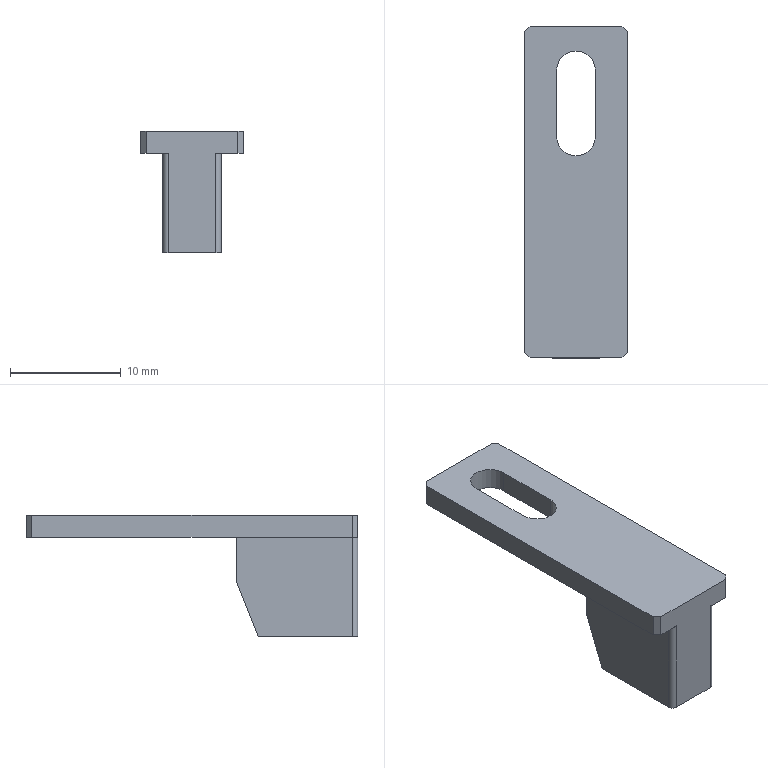Part | SolidWorks | features Chamfer 2, ICE 2, Extrusion 1, Fillet 1 | 1 solid | 21 faces | box 9.3 x 30 x 11 mm | volume 992.992 mm3 | plane 17 | cylinder 4 | commonest cylinder face diameters 1 x2 3.5 x2
STEP:
#1=CARTESIAN_POINT('',(2.65,-5.,0.));
#2=VERTEX_POINT('',#1);
#3=CARTESIAN_POINT('',(2.65,3.5,0.));
#4=VERTEX_POINT('',#3);
#5=CARTESIAN_POINT('',(2.65,5.5,0.));
#6=DIRECTION('',(0.,1.,0.));
#7=VECTOR('',#6,1000.);
#8=LINE('',#5,#7);
#9=EDGE_CURVE('',#2,#4,#8,.T.);
#10=ORIENTED_EDGE('',*,*,#9,.T.);
#11=CARTESIAN_POINT('',(2.65,5.5,5.));
#12=VERTEX_POINT('',#11);
#13=CARTESIAN_POINT('',(2.65,5.5,5.));
#14=DIRECTION('',(0.,0.3714,0.9285));
#15=VECTOR('',#14,1000.);
#16=LINE('',#13,#15);
#17=EDGE_CURVE('',#4,#12,#16,.T.);
#18=ORIENTED_EDGE('',*,*,#17,.T.);
#19=CARTESIAN_POINT('',(2.65,5.5,9.));
#20=VERTEX_POINT('',#19);
#21=CARTESIAN_POINT('',(2.65,5.5,9.));
#22=DIRECTION('',(0.,0.,-1.));
#23=VECTOR('',#22,1000.);
#24=LINE('',#21,#23);
#25=EDGE_CURVE('',#20,#12,#24,.T.);
#26=ORIENTED_EDGE('',*,*,#25,.F.);
#27=CARTESIAN_POINT('',(2.65,-5.,9.));
#28=VERTEX_POINT('',#27);
#29=CARTESIAN_POINT('',(2.65,5.5,9.));
#30=DIRECTION('',(0.,1.,0.));
#31=VECTOR('',#30,1000.);
#32=LINE('',#29,#31);
#33=EDGE_CURVE('',#28,#20,#32,.T.);
#34=ORIENTED_EDGE('',*,*,#33,.F.);
#35=CARTESIAN_POINT('',(2.65,-5.,9.));
#36=DIRECTION('',(0.,0.,-1.));
#37=VECTOR('',#36,1000.);
#38=LINE('',#35,#37);
#39=EDGE_CURVE('',#28,#2,#38,.T.);
#40=ORIENTED_EDGE('',*,*,#39,.T.);
#41=EDGE_LOOP('',(#10,#18,#26,#34,#40));
#42=FACE_OUTER_BOUND('',#41,.T.);
#43=CARTESIAN_POINT('',(2.65,5.5,9.));
#44=DIRECTION('',(-1.,0.,0.));
#45=DIRECTION('',(0.,-1.,0.));
#46=AXIS2_PLACEMENT_3D('',#43,#44,#45);
#47=PLANE('',#46);
#48=ADVANCED_FACE('',(#42),#47,.F.);
#49=ORIENTED_EDGE('',*,*,#25,.T.);
#50=CARTESIAN_POINT('',(-2.65,5.5,5.));
#51=VERTEX_POINT('',#50);
#52=CARTESIAN_POINT('',(-2.65,5.5,5.));
#53=DIRECTION('',(-1.,0.,0.));
#54=VECTOR('',#53,1000.);
#55=LINE('',#52,#54);
#56=EDGE_CURVE('',#12,#51,#55,.T.);
#57=ORIENTED_EDGE('',*,*,#56,.T.);
#58=CARTESIAN_POINT('',(-2.65,5.5,9.));
#59=VERTEX_POINT('',#58);
#60=CARTESIAN_POINT('',(-2.65,5.5,9.));
#61=DIRECTION('',(0.,0.,-1.));
#62=VECTOR('',#61,1000.);
#63=LINE('',#60,#62);
#64=EDGE_CURVE('',#59,#51,#63,.T.);
#65=ORIENTED_EDGE('',*,*,#64,.F.);
#66=CARTESIAN_POINT('',(-2.65,5.5,9.));
#67=DIRECTION('',(-1.,0.,0.));
#68=VECTOR('',#67,1000.);
#69=LINE('',#66,#68);
#70=EDGE_CURVE('',#20,#59,#69,.T.);
#71=ORIENTED_EDGE('',*,*,#70,.F.);
#72=EDGE_LOOP('',(#49,#57,#65,#71));
#73=FACE_OUTER_BOUND('',#72,.T.);
#74=CARTESIAN_POINT('',(-2.65,5.5,9.));
#75=DIRECTION('',(0.,-1.,0.));
#76=DIRECTION('',(0.,0.,-1.));
#77=AXIS2_PLACEMENT_3D('',#74,#75,#76);
#78=PLANE('',#77);
#79=ADVANCED_FACE('',(#73),#78,.F.);
#80=ORIENTED_EDGE('',*,*,#64,.T.);
#81=CARTESIAN_POINT('',(-2.65,3.5,0.));
#82=VERTEX_POINT('',#81);
#83=CARTESIAN_POINT('',(-2.65,5.5,5.));
#84=DIRECTION('',(0.,-0.3714,-0.9285));
#85=VECTOR('',#84,1000.);
#86=LINE('',#83,#85);
#87=EDGE_CURVE('',#51,#82,#86,.T.);
#88=ORIENTED_EDGE('',*,*,#87,.T.);
#89=CARTESIAN_POINT('',(-2.65,-5.,0.));
#90=VERTEX_POINT('',#89);
#91=CARTESIAN_POINT('',(-2.65,5.5,0.));
#92=DIRECTION('',(0.,-1.,0.));
#93=VECTOR('',#92,1000.);
#94=LINE('',#91,#93);
#95=EDGE_CURVE('',#82,#90,#94,.T.);
#96=ORIENTED_EDGE('',*,*,#95,.T.);
#97=CARTESIAN_POINT('',(-2.65,-5.,9.));
#98=VERTEX_POINT('',#97);
#99=CARTESIAN_POINT('',(-2.65,-5.,9.));
#100=DIRECTION('',(0.,0.,1.));
#101=VECTOR('',#100,1000.);
#102=LINE('',#99,#101);
#103=EDGE_CURVE('',#90,#98,#102,.T.);
#104=ORIENTED_EDGE('',*,*,#103,.T.);
#105=CARTESIAN_POINT('',(-2.65,5.5,9.));
#106=DIRECTION('',(0.,-1.,0.));
#107=VECTOR('',#106,1000.);
#108=LINE('',#105,#107);
#109=EDGE_CURVE('',#59,#98,#108,.T.);
#110=ORIENTED_EDGE('',*,*,#109,.F.);
#111=EDGE_LOOP('',(#80,#88,#96,#104,#110));
#112=FACE_OUTER_BOUND('',#111,.T.);
#113=CARTESIAN_POINT('',(-2.65,5.5,9.));
#114=DIRECTION('',(1.,0.,0.));
#115=DIRECTION('',(0.,1.,0.));
#116=AXIS2_PLACEMENT_3D('',#113,#114,#115);
#117=PLANE('',#116);
#118=ADVANCED_FACE('',(#112),#117,.F.);
#119=CARTESIAN_POINT('',(-2.15,-5.5,0.));
#120=VERTEX_POINT('',#119);
#121=CARTESIAN_POINT('',(2.15,-5.5,0.));
#122=VERTEX_POINT('',#121);
#123=CARTESIAN_POINT('',(-2.65,-5.5,0.));
#124=DIRECTION('',(1.,0.,0.));
#125=VECTOR('',#124,1000.);
#126=LINE('',#123,#125);
#127=EDGE_CURVE('',#120,#122,#126,.T.);
#128=ORIENTED_EDGE('',*,*,#127,.T.);
#129=CARTESIAN_POINT('',(2.15,-5.5,9.));
#130=VERTEX_POINT('',#129);
#131=CARTESIAN_POINT('',(2.15,-5.5,9.));
#132=DIRECTION('',(0.,0.,1.));
#133=VECTOR('',#132,1000.);
#134=LINE('',#131,#133);
#135=EDGE_CURVE('',#122,#130,#134,.T.);
#136=ORIENTED_EDGE('',*,*,#135,.T.);
#137=CARTESIAN_POINT('',(4.15,-5.5,9.));
#138=VERTEX_POINT('',#137);
#139=CARTESIAN_POINT('',(4.65,-5.5,9.));
#140=DIRECTION('',(1.,0.,0.));
#141=VECTOR('',#140,1000.);
#142=LINE('',#139,#141);
#143=EDGE_CURVE('',#130,#138,#142,.T.);
#144=ORIENTED_EDGE('',*,*,#143,.T.);
#145=CARTESIAN_POINT('',(4.15,-5.5,11.));
#146=VERTEX_POINT('',#145);
#147=CARTESIAN_POINT('',(4.15,-5.5,9.));
#148=DIRECTION('',(0.,0.,1.));
#149=VECTOR('',#148,1000.);
#150=LINE('',#147,#149);
#151=EDGE_CURVE('',#138,#146,#150,.T.);
#152=ORIENTED_EDGE('',*,*,#151,.T.);
#153=CARTESIAN_POINT('',(-4.15,-5.5,11.));
#154=VERTEX_POINT('',#153);
#155=CARTESIAN_POINT('',(4.65,-5.5,11.));
#156=DIRECTION('',(1.,0.,0.));
#157=VECTOR('',#156,1000.);
#158=LINE('',#155,#157);
#159=EDGE_CURVE('',#154,#146,#158,.T.);
#160=ORIENTED_EDGE('',*,*,#159,.F.);
#161=CARTESIAN_POINT('',(-4.15,-5.5,9.));
#162=VERTEX_POINT('',#161);
#163=CARTESIAN_POINT('',(-4.15,-5.5,9.));
#164=DIRECTION('',(0.,0.,-1.));
#165=VECTOR('',#164,1000.);
#166=LINE('',#163,#165);
#167=EDGE_CURVE('',#154,#162,#166,.T.);
#168=ORIENTED_EDGE('',*,*,#167,.T.);
#169=CARTESIAN_POINT('',(-2.15,-5.5,9.));
#170=VERTEX_POINT('',#169);
#171=CARTESIAN_POINT('',(4.65,-5.5,9.));
#172=DIRECTION('',(1.,0.,0.));
#173=VECTOR('',#172,1000.);
#174=LINE('',#171,#173);
#175=EDGE_CURVE('',#162,#170,#174,.T.);
#176=ORIENTED_EDGE('',*,*,#175,.T.);
#177=CARTESIAN_POINT('',(-2.15,-5.5,9.));
#178=DIRECTION('',(0.,0.,-1.));
#179=VECTOR('',#178,1000.);
#180=LINE('',#177,#179);
#181=EDGE_CURVE('',#170,#120,#180,.T.);
#182=ORIENTED_EDGE('',*,*,#181,.T.);
#183=EDGE_LOOP('',(#128,#136,#144,#152,#160,#168,#176,#182));
#184=FACE_OUTER_BOUND('',#183,.T.);
#185=CARTESIAN_POINT('',(-2.65,-5.5,9.));
#186=DIRECTION('',(0.,1.,0.));
#187=DIRECTION('',(0.,0.,1.));
#188=AXIS2_PLACEMENT_3D('',#185,#186,#187);
#189=PLANE('',#188);
#190=ADVANCED_FACE('',(#184),#189,.F.);
#191=ORIENTED_EDGE('',*,*,#95,.F.);
#192=CARTESIAN_POINT('',(0.,3.5,0.));
#193=DIRECTION('',(1.,0.,0.));
#194=VECTOR('',#193,1000.);
#195=LINE('',#192,#194);
#196=EDGE_CURVE('',#82,#4,#195,.T.);
#197=ORIENTED_EDGE('',*,*,#196,.T.);
#198=ORIENTED_EDGE('',*,*,#9,.F.);
#199=CARTESIAN_POINT('',(2.15,-5.,0.));
#200=DIRECTION('',(0.,0.,-1.));
#201=DIRECTION('',(1.,0.,0.));
#202=AXIS2_PLACEMENT_3D('',#199,#200,#201);
#203=CIRCLE('',#202,0.5);
#204=EDGE_CURVE('',#2,#122,#203,.T.);
#205=ORIENTED_EDGE('',*,*,#204,.T.);
#206=ORIENTED_EDGE('',*,*,#127,.F.);
#207=CARTESIAN_POINT('',(-2.15,-5.,0.));
#208=DIRECTION('',(0.,0.,-1.));
#209=DIRECTION('',(1.,0.,0.));
#210=AXIS2_PLACEMENT_3D('',#207,#208,#209);
#211=CIRCLE('',#210,0.5);
#212=EDGE_CURVE('',#120,#90,#211,.T.);
#213=ORIENTED_EDGE('',*,*,#212,.T.);
#214=EDGE_LOOP('',(#191,#197,#198,#205,#206,#213));
#215=FACE_OUTER_BOUND('',#214,.T.);
#216=CARTESIAN_POINT('',(0.,0.,0.));
#217=DIRECTION('',(0.,0.,1.));
#218=DIRECTION('',(1.,0.,0.));
#219=AXIS2_PLACEMENT_3D('',#216,#217,#218);
#220=PLANE('',#219);
#221=ADVANCED_FACE('',(#215),#220,.F.);
#222=CARTESIAN_POINT('',(1.75,14.5,9.));
#223=VERTEX_POINT('',#222);
#224=CARTESIAN_POINT('',(1.75,20.5,9.));
#225=VERTEX_POINT('',#224);
#226=CARTESIAN_POINT('',(1.75,0.,9.));
#227=DIRECTION('',(0.,1.,0.));
#228=VECTOR('',#227,1000.);
#229=LINE('',#226,#228);
#230=EDGE_CURVE('',#223,#225,#229,.T.);
#231=ORIENTED_EDGE('',*,*,#230,.T.);
#232=CARTESIAN_POINT('',(-1.75,20.5,9.));
#233=VERTEX_POINT('',#232);
#234=CARTESIAN_POINT('',(0.,20.5,9.));
#235=DIRECTION('',(0.,0.,1.));
#236=DIRECTION('',(1.,0.,0.));
#237=AXIS2_PLACEMENT_3D('',#234,#235,#236);
#238=CIRCLE('',#237,1.75);
#239=EDGE_CURVE('',#225,#233,#238,.T.);
#240=ORIENTED_EDGE('',*,*,#239,.T.);
#241=CARTESIAN_POINT('',(-1.75,14.5,9.));
#242=VERTEX_POINT('',#241);
#243=CARTESIAN_POINT('',(-1.75,0.,9.));
#244=DIRECTION('',(0.,-1.,0.));
#245=VECTOR('',#244,1000.);
#246=LINE('',#243,#245);
#247=EDGE_CURVE('',#233,#242,#246,.T.);
#248=ORIENTED_EDGE('',*,*,#247,.T.);
#249=CARTESIAN_POINT('',(0.,14.5,9.));
#250=DIRECTION('',(0.,0.,1.));
#251=DIRECTION('',(1.,0.,0.));
#252=AXIS2_PLACEMENT_3D('',#249,#250,#251);
#253=CIRCLE('',#252,1.75);
#254=EDGE_CURVE('',#242,#223,#253,.T.);
#255=ORIENTED_EDGE('',*,*,#254,.T.);
#256=EDGE_LOOP('',(#231,#240,#248,#255));
#257=FACE_BOUND('',#256,.T.);
#258=ORIENTED_EDGE('',*,*,#175,.F.);
#259=CARTESIAN_POINT('',(-4.65,-5.,9.));
#260=VERTEX_POINT('',#259);
#261=CARTESIAN_POINT('',(-4.15,-5.5,9.));
#262=DIRECTION('',(-0.7071,0.7071,0.));
#263=VECTOR('',#262,1000.);
#264=LINE('',#261,#263);
#265=EDGE_CURVE('',#162,#260,#264,.T.);
#266=ORIENTED_EDGE('',*,*,#265,.T.);
#267=CARTESIAN_POINT('',(-4.65,24.,9.));
#268=VERTEX_POINT('',#267);
#269=CARTESIAN_POINT('',(-4.65,-5.5,9.));
#270=DIRECTION('',(0.,-1.,0.));
#271=VECTOR('',#270,1000.);
#272=LINE('',#269,#271);
#273=EDGE_CURVE('',#268,#260,#272,.T.);
#274=ORIENTED_EDGE('',*,*,#273,.F.);
#275=CARTESIAN_POINT('',(-4.15,24.5,9.));
#276=VERTEX_POINT('',#275);
#277=CARTESIAN_POINT('',(-4.65,24.,9.));
#278=DIRECTION('',(0.7071,0.7071,0.));
#279=VECTOR('',#278,1000.);
#280=LINE('',#277,#279);
#281=EDGE_CURVE('',#268,#276,#280,.T.);
#282=ORIENTED_EDGE('',*,*,#281,.T.);
#283=CARTESIAN_POINT('',(4.15,24.5,9.));
#284=VERTEX_POINT('',#283);
#285=CARTESIAN_POINT('',(4.65,24.5,9.));
#286=DIRECTION('',(-1.,0.,0.));
#287=VECTOR('',#286,1000.);
#288=LINE('',#285,#287);
#289=EDGE_CURVE('',#284,#276,#288,.T.);
#290=ORIENTED_EDGE('',*,*,#289,.F.);
#291=CARTESIAN_POINT('',(4.65,24.,9.));
#292=VERTEX_POINT('',#291);
#293=CARTESIAN_POINT('',(4.15,24.5,9.));
#294=DIRECTION('',(0.7071,-0.7071,0.));
#295=VECTOR('',#294,1000.);
#296=LINE('',#293,#295);
#297=EDGE_CURVE('',#284,#292,#296,.T.);
#298=ORIENTED_EDGE('',*,*,#297,.T.);
#299=CARTESIAN_POINT('',(4.65,-5.,9.));
#300=VERTEX_POINT('',#299);
#301=CARTESIAN_POINT('',(4.65,-5.5,9.));
#302=DIRECTION('',(0.,1.,0.));
#303=VECTOR('',#302,1000.);
#304=LINE('',#301,#303);
#305=EDGE_CURVE('',#300,#292,#304,.T.);
#306=ORIENTED_EDGE('',*,*,#305,.F.);
#307=CARTESIAN_POINT('',(4.65,-5.,9.));
#308=DIRECTION('',(-0.7071,-0.7071,0.));
#309=VECTOR('',#308,1000.);
#310=LINE('',#307,#309);
#311=EDGE_CURVE('',#300,#138,#310,.T.);
#312=ORIENTED_EDGE('',*,*,#311,.T.);
#313=ORIENTED_EDGE('',*,*,#143,.F.);
#314=CARTESIAN_POINT('',(2.15,-5.,9.));
#315=DIRECTION('',(0.,0.,1.));
#316=DIRECTION('',(1.,0.,0.));
#317=AXIS2_PLACEMENT_3D('',#314,#315,#316);
#318=CIRCLE('',#317,0.5);
#319=EDGE_CURVE('',#130,#28,#318,.T.);
#320=ORIENTED_EDGE('',*,*,#319,.T.);
#321=ORIENTED_EDGE('',*,*,#33,.T.);
#322=ORIENTED_EDGE('',*,*,#70,.T.);
#323=ORIENTED_EDGE('',*,*,#109,.T.);
#324=CARTESIAN_POINT('',(-2.15,-5.,9.));
#325=DIRECTION('',(0.,0.,1.));
#326=DIRECTION('',(1.,0.,0.));
#327=AXIS2_PLACEMENT_3D('',#324,#325,#326);
#328=CIRCLE('',#327,0.5);
#329=EDGE_CURVE('',#98,#170,#328,.T.);
#330=ORIENTED_EDGE('',*,*,#329,.T.);
#331=EDGE_LOOP('',(#258,#266,#274,#282,#290,#298,#306,#312,#313,#320,#321,#322,#323,#330));
#332=FACE_OUTER_BOUND('',#331,.T.);
#333=CARTESIAN_POINT('',(0.,0.,9.));
#334=DIRECTION('',(0.,0.,1.));
#335=DIRECTION('',(1.,0.,0.));
#336=AXIS2_PLACEMENT_3D('',#333,#334,#335);
#337=PLANE('',#336);
#338=ADVANCED_FACE('',(#257,#332),#337,.F.);
#339=CARTESIAN_POINT('',(4.65,-5.,11.));
#340=VERTEX_POINT('',#339);
#341=CARTESIAN_POINT('',(4.65,24.,11.));
#342=VERTEX_POINT('',#341);
#343=CARTESIAN_POINT('',(4.65,-5.5,11.));
#344=DIRECTION('',(0.,1.,0.));
#345=VECTOR('',#344,1000.);
#346=LINE('',#343,#345);
#347=EDGE_CURVE('',#340,#342,#346,.T.);
#348=ORIENTED_EDGE('',*,*,#347,.F.);
#349=CARTESIAN_POINT('',(4.65,-5.,11.));
#350=DIRECTION('',(0.,0.,-1.));
#351=VECTOR('',#350,1000.);
#352=LINE('',#349,#351);
#353=EDGE_CURVE('',#340,#300,#352,.T.);
#354=ORIENTED_EDGE('',*,*,#353,.T.);
#355=ORIENTED_EDGE('',*,*,#305,.T.);
#356=CARTESIAN_POINT('',(4.65,24.,11.));
#357=DIRECTION('',(0.,0.,1.));
#358=VECTOR('',#357,1000.);
#359=LINE('',#356,#358);
#360=EDGE_CURVE('',#292,#342,#359,.T.);
#361=ORIENTED_EDGE('',*,*,#360,.T.);
#362=EDGE_LOOP('',(#348,#354,#355,#361));
#363=FACE_OUTER_BOUND('',#362,.T.);
#364=CARTESIAN_POINT('',(4.65,-5.5,11.));
#365=DIRECTION('',(-1.,0.,0.));
#366=DIRECTION('',(0.,-1.,0.));
#367=AXIS2_PLACEMENT_3D('',#364,#365,#366);
#368=PLANE('',#367);
#369=ADVANCED_FACE('',(#363),#368,.F.);
#370=CARTESIAN_POINT('',(4.15,24.5,11.));
#371=VERTEX_POINT('',#370);
#372=CARTESIAN_POINT('',(-4.15,24.5,11.));
#373=VERTEX_POINT('',#372);
#374=CARTESIAN_POINT('',(4.65,24.5,11.));
#375=DIRECTION('',(-1.,0.,0.));
#376=VECTOR('',#375,1000.);
#377=LINE('',#374,#376);
#378=EDGE_CURVE('',#371,#373,#377,.T.);
#379=ORIENTED_EDGE('',*,*,#378,.F.);
#380=CARTESIAN_POINT('',(4.15,24.5,11.));
#381=DIRECTION('',(0.,0.,-1.));
#382=VECTOR('',#381,1000.);
#383=LINE('',#380,#382);
#384=EDGE_CURVE('',#371,#284,#383,.T.);
#385=ORIENTED_EDGE('',*,*,#384,.T.);
#386=ORIENTED_EDGE('',*,*,#289,.T.);
#387=CARTESIAN_POINT('',(-4.15,24.5,11.));
#388=DIRECTION('',(0.,0.,1.));
#389=VECTOR('',#388,1000.);
#390=LINE('',#387,#389);
#391=EDGE_CURVE('',#276,#373,#390,.T.);
#392=ORIENTED_EDGE('',*,*,#391,.T.);
#393=EDGE_LOOP('',(#379,#385,#386,#392));
#394=FACE_OUTER_BOUND('',#393,.T.);
#395=CARTESIAN_POINT('',(4.65,24.5,11.));
#396=DIRECTION('',(0.,-1.,0.));
#397=DIRECTION('',(0.,0.,-1.));
#398=AXIS2_PLACEMENT_3D('',#395,#396,#397);
#399=PLANE('',#398);
#400=ADVANCED_FACE('',(#394),#399,.F.);
#401=ORIENTED_EDGE('',*,*,#273,.T.);
#402=CARTESIAN_POINT('',(-4.65,-5.,11.));
#403=VERTEX_POINT('',#402);
#404=CARTESIAN_POINT('',(-4.65,-5.,11.));
#405=DIRECTION('',(0.,0.,1.));
#406=VECTOR('',#405,1000.);
#407=LINE('',#404,#406);
#408=EDGE_CURVE('',#260,#403,#407,.T.);
#409=ORIENTED_EDGE('',*,*,#408,.T.);
#410=CARTESIAN_POINT('',(-4.65,24.,11.));
#411=VERTEX_POINT('',#410);
#412=CARTESIAN_POINT('',(-4.65,-5.5,11.));
#413=DIRECTION('',(0.,-1.,0.));
#414=VECTOR('',#413,1000.);
#415=LINE('',#412,#414);
#416=EDGE_CURVE('',#411,#403,#415,.T.);
#417=ORIENTED_EDGE('',*,*,#416,.F.);
#418=CARTESIAN_POINT('',(-4.65,24.,11.));
#419=DIRECTION('',(0.,0.,-1.));
#420=VECTOR('',#419,1000.);
#421=LINE('',#418,#420);
#422=EDGE_CURVE('',#411,#268,#421,.T.);
#423=ORIENTED_EDGE('',*,*,#422,.T.);
#424=EDGE_LOOP('',(#401,#409,#417,#423));
#425=FACE_OUTER_BOUND('',#424,.T.);
#426=CARTESIAN_POINT('',(-4.65,-5.5,11.));
#427=DIRECTION('',(1.,0.,0.));
#428=DIRECTION('',(0.,0.,-1.));
#429=AXIS2_PLACEMENT_3D('',#426,#427,#428);
#430=PLANE('',#429);
#431=ADVANCED_FACE('',(#425),#430,.F.);
#432=CARTESIAN_POINT('',(1.75,20.5,11.));
#433=VERTEX_POINT('',#432);
#434=CARTESIAN_POINT('',(-1.75,20.5,11.));
#435=VERTEX_POINT('',#434);
#436=CARTESIAN_POINT('',(0.,20.5,11.));
#437=DIRECTION('',(0.,0.,1.));
#438=DIRECTION('',(1.,0.,0.));
#439=AXIS2_PLACEMENT_3D('',#436,#437,#438);
#440=CIRCLE('',#439,1.75);
#441=EDGE_CURVE('',#433,#435,#440,.T.);
#442=ORIENTED_EDGE('',*,*,#441,.F.);
#443=CARTESIAN_POINT('',(1.75,14.5,11.));
#444=VERTEX_POINT('',#443);
#445=CARTESIAN_POINT('',(1.75,20.5,11.));
#446=DIRECTION('',(0.,1.,0.));
#447=VECTOR('',#446,1000.);
#448=LINE('',#445,#447);
#449=EDGE_CURVE('',#444,#433,#448,.T.);
#450=ORIENTED_EDGE('',*,*,#449,.F.);
#451=CARTESIAN_POINT('',(-1.75,14.5,11.));
#452=VERTEX_POINT('',#451);
#453=CARTESIAN_POINT('',(0.,14.5,11.));
#454=DIRECTION('',(0.,0.,1.));
#455=DIRECTION('',(1.,0.,0.));
#456=AXIS2_PLACEMENT_3D('',#453,#454,#455);
#457=CIRCLE('',#456,1.75);
#458=EDGE_CURVE('',#452,#444,#457,.T.);
#459=ORIENTED_EDGE('',*,*,#458,.F.);
#460=CARTESIAN_POINT('',(-1.75,20.5,11.));
#461=DIRECTION('',(0.,-1.,0.));
#462=VECTOR('',#461,1000.);
#463=LINE('',#460,#462);
#464=EDGE_CURVE('',#435,#452,#463,.T.);
#465=ORIENTED_EDGE('',*,*,#464,.F.);
#466=EDGE_LOOP('',(#442,#450,#459,#465));
#467=FACE_BOUND('',#466,.T.);
#468=ORIENTED_EDGE('',*,*,#416,.T.);
#469=CARTESIAN_POINT('',(-4.825,-4.825,11.));
#470=DIRECTION('',(0.7071,-0.7071,0.));
#471=VECTOR('',#470,1000.);
#472=LINE('',#469,#471);
#473=EDGE_CURVE('',#403,#154,#472,.T.);
#474=ORIENTED_EDGE('',*,*,#473,.T.);
#475=ORIENTED_EDGE('',*,*,#159,.T.);
#476=CARTESIAN_POINT('',(4.825,-4.825,11.));
#477=DIRECTION('',(0.7071,0.7071,0.));
#478=VECTOR('',#477,1000.);
#479=LINE('',#476,#478);
#480=EDGE_CURVE('',#146,#340,#479,.T.);
#481=ORIENTED_EDGE('',*,*,#480,.T.);
#482=ORIENTED_EDGE('',*,*,#347,.T.);
#483=CARTESIAN_POINT('',(14.325,14.325,11.));
#484=DIRECTION('',(-0.7071,0.7071,0.));
#485=VECTOR('',#484,1000.);
#486=LINE('',#483,#485);
#487=EDGE_CURVE('',#342,#371,#486,.T.);
#488=ORIENTED_EDGE('',*,*,#487,.T.);
#489=ORIENTED_EDGE('',*,*,#378,.T.);
#490=CARTESIAN_POINT('',(-14.325,14.325,11.));
#491=DIRECTION('',(-0.7071,-0.7071,0.));
#492=VECTOR('',#491,1000.);
#493=LINE('',#490,#492);
#494=EDGE_CURVE('',#373,#411,#493,.T.);
#495=ORIENTED_EDGE('',*,*,#494,.T.);
#496=EDGE_LOOP('',(#468,#474,#475,#481,#482,#488,#489,#495));
#497=FACE_OUTER_BOUND('',#496,.T.);
#498=CARTESIAN_POINT('',(0.,0.,11.));
#499=DIRECTION('',(0.,0.,1.));
#500=DIRECTION('',(1.,0.,0.));
#501=AXIS2_PLACEMENT_3D('',#498,#499,#500);
#502=PLANE('',#501);
#503=ADVANCED_FACE('',(#467,#497),#502,.T.);
#504=CARTESIAN_POINT('',(1.75,20.5,1.));
#505=DIRECTION('',(0.,0.,1.));
#506=VECTOR('',#505,1000.);
#507=LINE('',#504,#506);
#508=EDGE_CURVE('',#225,#433,#507,.T.);
#509=ORIENTED_EDGE('',*,*,#508,.T.);
#510=ORIENTED_EDGE('',*,*,#441,.T.);
#511=CARTESIAN_POINT('',(-1.75,20.5,1.));
#512=DIRECTION('',(0.,0.,1.));
#513=VECTOR('',#512,1000.);
#514=LINE('',#511,#513);
#515=EDGE_CURVE('',#233,#435,#514,.T.);
#516=ORIENTED_EDGE('',*,*,#515,.F.);
#517=ORIENTED_EDGE('',*,*,#239,.F.);
#518=EDGE_LOOP('',(#509,#510,#516,#517));
#519=FACE_OUTER_BOUND('',#518,.T.);
#520=CARTESIAN_POINT('',(0.,20.5,1.));
#521=DIRECTION('',(0.,0.,1.));
#522=DIRECTION('',(1.,0.,0.));
#523=AXIS2_PLACEMENT_3D('',#520,#521,#522);
#524=CYLINDRICAL_SURFACE('',#523,1.75);
#525=ADVANCED_FACE('',(#519),#524,.F.);
#526=CARTESIAN_POINT('',(1.75,14.5,1.));
#527=DIRECTION('',(0.,0.,1.));
#528=VECTOR('',#527,1000.);
#529=LINE('',#526,#528);
#530=EDGE_CURVE('',#223,#444,#529,.T.);
#531=ORIENTED_EDGE('',*,*,#530,.T.);
#532=ORIENTED_EDGE('',*,*,#449,.T.);
#533=ORIENTED_EDGE('',*,*,#508,.F.);
#534=ORIENTED_EDGE('',*,*,#230,.F.);
#535=EDGE_LOOP('',(#531,#532,#533,#534));
#536=FACE_OUTER_BOUND('',#535,.T.);
#537=CARTESIAN_POINT('',(1.75,20.5,1.));
#538=DIRECTION('',(1.,0.,0.));
#539=DIRECTION('',(0.,1.,0.));
#540=AXIS2_PLACEMENT_3D('',#537,#538,#539);
#541=PLANE('',#540);
#542=ADVANCED_FACE('',(#536),#541,.F.);
#543=CARTESIAN_POINT('',(-1.75,14.5,1.));
#544=DIRECTION('',(0.,0.,1.));
#545=VECTOR('',#544,1000.);
#546=LINE('',#543,#545);
#547=EDGE_CURVE('',#242,#452,#546,.T.);
#548=ORIENTED_EDGE('',*,*,#547,.T.);
#549=ORIENTED_EDGE('',*,*,#458,.T.);
#550=ORIENTED_EDGE('',*,*,#530,.F.);
#551=ORIENTED_EDGE('',*,*,#254,.F.);
#552=EDGE_LOOP('',(#548,#549,#550,#551));
#553=FACE_OUTER_BOUND('',#552,.T.);
#554=CARTESIAN_POINT('',(0.,14.5,1.));
#555=DIRECTION('',(0.,0.,1.));
#556=DIRECTION('',(1.,0.,0.));
#557=AXIS2_PLACEMENT_3D('',#554,#555,#556);
#558=CYLINDRICAL_SURFACE('',#557,1.75);
#559=ADVANCED_FACE('',(#553),#558,.F.);
#560=ORIENTED_EDGE('',*,*,#515,.T.);
#561=ORIENTED_EDGE('',*,*,#464,.T.);
#562=ORIENTED_EDGE('',*,*,#547,.F.);
#563=ORIENTED_EDGE('',*,*,#247,.F.);
#564=EDGE_LOOP('',(#560,#561,#562,#563));
#565=FACE_OUTER_BOUND('',#564,.T.);
#566=CARTESIAN_POINT('',(-1.75,20.5,1.));
#567=DIRECTION('',(-1.,0.,0.));
#568=DIRECTION('',(0.,-1.,0.));
#569=AXIS2_PLACEMENT_3D('',#566,#567,#568);
#570=PLANE('',#569);
#571=ADVANCED_FACE('',(#565),#570,.F.);
#572=ORIENTED_EDGE('',*,*,#473,.F.);
#573=ORIENTED_EDGE('',*,*,#408,.F.);
#574=ORIENTED_EDGE('',*,*,#265,.F.);
#575=ORIENTED_EDGE('',*,*,#167,.F.);
#576=EDGE_LOOP('',(#572,#573,#574,#575));
#577=FACE_OUTER_BOUND('',#576,.T.);
#578=CARTESIAN_POINT('',(-4.15,-5.5,9.));
#579=DIRECTION('',(0.7071,0.7071,0.));
#580=DIRECTION('',(0.,0.,-1.));
#581=AXIS2_PLACEMENT_3D('',#578,#579,#580);
#582=PLANE('',#581);
#583=ADVANCED_FACE('',(#577),#582,.F.);
#584=ORIENTED_EDGE('',*,*,#480,.F.);
#585=ORIENTED_EDGE('',*,*,#151,.F.);
#586=ORIENTED_EDGE('',*,*,#311,.F.);
#587=ORIENTED_EDGE('',*,*,#353,.F.);
#588=EDGE_LOOP('',(#584,#585,#586,#587));
#589=FACE_OUTER_BOUND('',#588,.T.);
#590=CARTESIAN_POINT('',(4.65,-5.,11.));
#591=DIRECTION('',(-0.7071,0.7071,0.));
#592=DIRECTION('',(0.,0.,-1.));
#593=AXIS2_PLACEMENT_3D('',#590,#591,#592);
#594=PLANE('',#593);
#595=ADVANCED_FACE('',(#589),#594,.F.);
#596=ORIENTED_EDGE('',*,*,#487,.F.);
#597=ORIENTED_EDGE('',*,*,#360,.F.);
#598=ORIENTED_EDGE('',*,*,#297,.F.);
#599=ORIENTED_EDGE('',*,*,#384,.F.);
#600=EDGE_LOOP('',(#596,#597,#598,#599));
#601=FACE_OUTER_BOUND('',#600,.T.);
#602=CARTESIAN_POINT('',(4.15,24.5,11.));
#603=DIRECTION('',(-0.7071,-0.7071,0.));
#604=DIRECTION('',(0.,0.,-1.));
#605=AXIS2_PLACEMENT_3D('',#602,#603,#604);
#606=PLANE('',#605);
#607=ADVANCED_FACE('',(#601),#606,.F.);
#608=ORIENTED_EDGE('',*,*,#494,.F.);
#609=ORIENTED_EDGE('',*,*,#391,.F.);
#610=ORIENTED_EDGE('',*,*,#281,.F.);
#611=ORIENTED_EDGE('',*,*,#422,.F.);
#612=EDGE_LOOP('',(#608,#609,#610,#611));
#613=FACE_OUTER_BOUND('',#612,.T.);
#614=CARTESIAN_POINT('',(-4.65,24.,11.));
#615=DIRECTION('',(0.7071,-0.7071,0.));
#616=DIRECTION('',(0.,0.,-1.));
#617=AXIS2_PLACEMENT_3D('',#614,#615,#616);
#618=PLANE('',#617);
#619=ADVANCED_FACE('',(#613),#618,.F.);
#620=ORIENTED_EDGE('',*,*,#319,.F.);
#621=ORIENTED_EDGE('',*,*,#135,.F.);
#622=ORIENTED_EDGE('',*,*,#204,.F.);
#623=ORIENTED_EDGE('',*,*,#39,.F.);
#624=EDGE_LOOP('',(#620,#621,#622,#623));
#625=FACE_OUTER_BOUND('',#624,.T.);
#626=CARTESIAN_POINT('',(2.15,-5.,9.));
#627=DIRECTION('',(0.,0.,-1.));
#628=DIRECTION('',(-1.,0.,0.));
#629=AXIS2_PLACEMENT_3D('',#626,#627,#628);
#630=CYLINDRICAL_SURFACE('',#629,0.5);
#631=ADVANCED_FACE('',(#625),#630,.T.);
#632=ORIENTED_EDGE('',*,*,#329,.F.);
#633=ORIENTED_EDGE('',*,*,#103,.F.);
#634=ORIENTED_EDGE('',*,*,#212,.F.);
#635=ORIENTED_EDGE('',*,*,#181,.F.);
#636=EDGE_LOOP('',(#632,#633,#634,#635));
#637=FACE_OUTER_BOUND('',#636,.T.);
#638=CARTESIAN_POINT('',(-2.15,-5.,9.));
#639=DIRECTION('',(0.,0.,-1.));
#640=DIRECTION('',(-1.,0.,0.));
#641=AXIS2_PLACEMENT_3D('',#638,#639,#640);
#642=CYLINDRICAL_SURFACE('',#641,0.5);
#643=ADVANCED_FACE('',(#637),#642,.T.);
#644=ORIENTED_EDGE('',*,*,#17,.F.);
#645=ORIENTED_EDGE('',*,*,#196,.F.);
#646=ORIENTED_EDGE('',*,*,#87,.F.);
#647=ORIENTED_EDGE('',*,*,#56,.F.);
#648=EDGE_LOOP('',(#644,#645,#646,#647));
#649=FACE_OUTER_BOUND('',#648,.T.);
#650=CARTESIAN_POINT('',(-2.65,5.5,5.));
#651=DIRECTION('',(0.,-0.9285,0.3714));
#652=DIRECTION('',(-1.,0.,0.));
#653=AXIS2_PLACEMENT_3D('',#650,#651,#652);
#654=PLANE('',#653);
#655=ADVANCED_FACE('',(#649),#654,.F.);
#656=CLOSED_SHELL('',(#48,#79,#118,#190,#221,#338,#369,#400,#431,#503,#525,#542,#559,#571,#583,#595,#607,#619,#631,#643,#655));
#657=MANIFOLD_SOLID_BREP('',#656);
#658=CARTESIAN_POINT('',(0.,0.,0.));
#659=DIRECTION('',(0.,0.,1.));
#660=DIRECTION('',(1.,0.,0.));
#661=AXIS2_PLACEMENT_3D('',#658,#659,#660);
#662=(LENGTH_UNIT()NAMED_UNIT(*)SI_UNIT(.MILLI.,.METRE.));
#663=UNCERTAINTY_MEASURE_WITH_UNIT(LENGTH_MEASURE(0.00001),#662,'','');
#664=(NAMED_UNIT(*)PLANE_ANGLE_UNIT()SI_UNIT($,.RADIAN.));
#665=(NAMED_UNIT(*)SI_UNIT($,.STERADIAN.)SOLID_ANGLE_UNIT());
#666=(GEOMETRIC_REPRESENTATION_CONTEXT(3)GLOBAL_UNCERTAINTY_ASSIGNED_CONTEXT((#663))GLOBAL_UNIT_ASSIGNED_CONTEXT((#662,#664,#665))REPRESENTATION_CONTEXT('',''));
#667=ADVANCED_BREP_SHAPE_REPRESENTATION('',(#657,#661),#666);